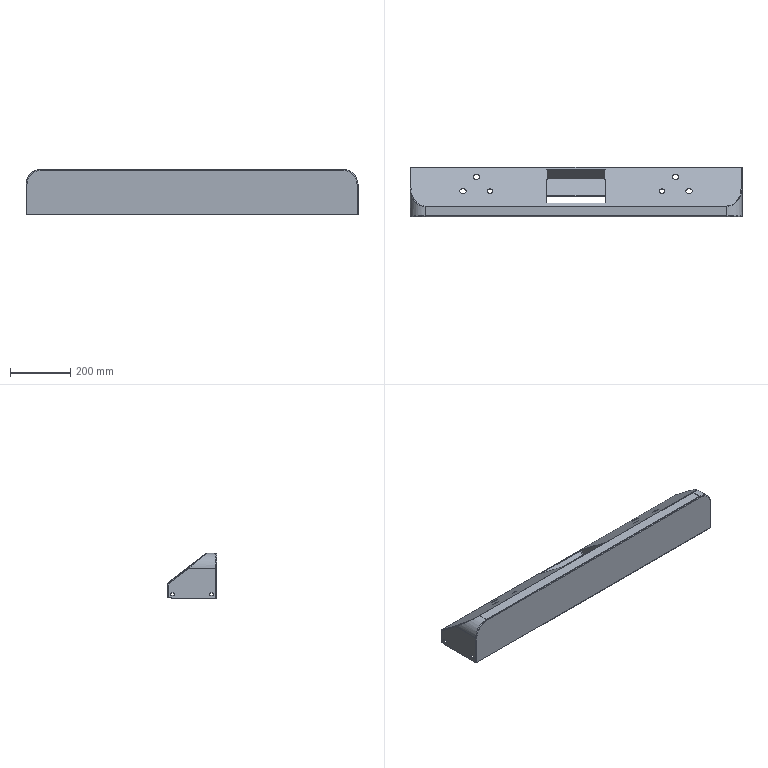Part | SolidWorks | features ICE 7, Fillet 3, Cut 1, Extrusion 1, HoleWzd 1, MoveFace 1, Shell 1 | 1 solid | 89 faces | box 1100 x 165 x 150 mm | volume 712221 mm3 | cylinder 43 | plane 40 | torus 2 | sphere 2 | spline 2 | commonest cylinder face diameters 6 x13 8 x8 22.5 x8 9 x4 19.5 x4 20 x2